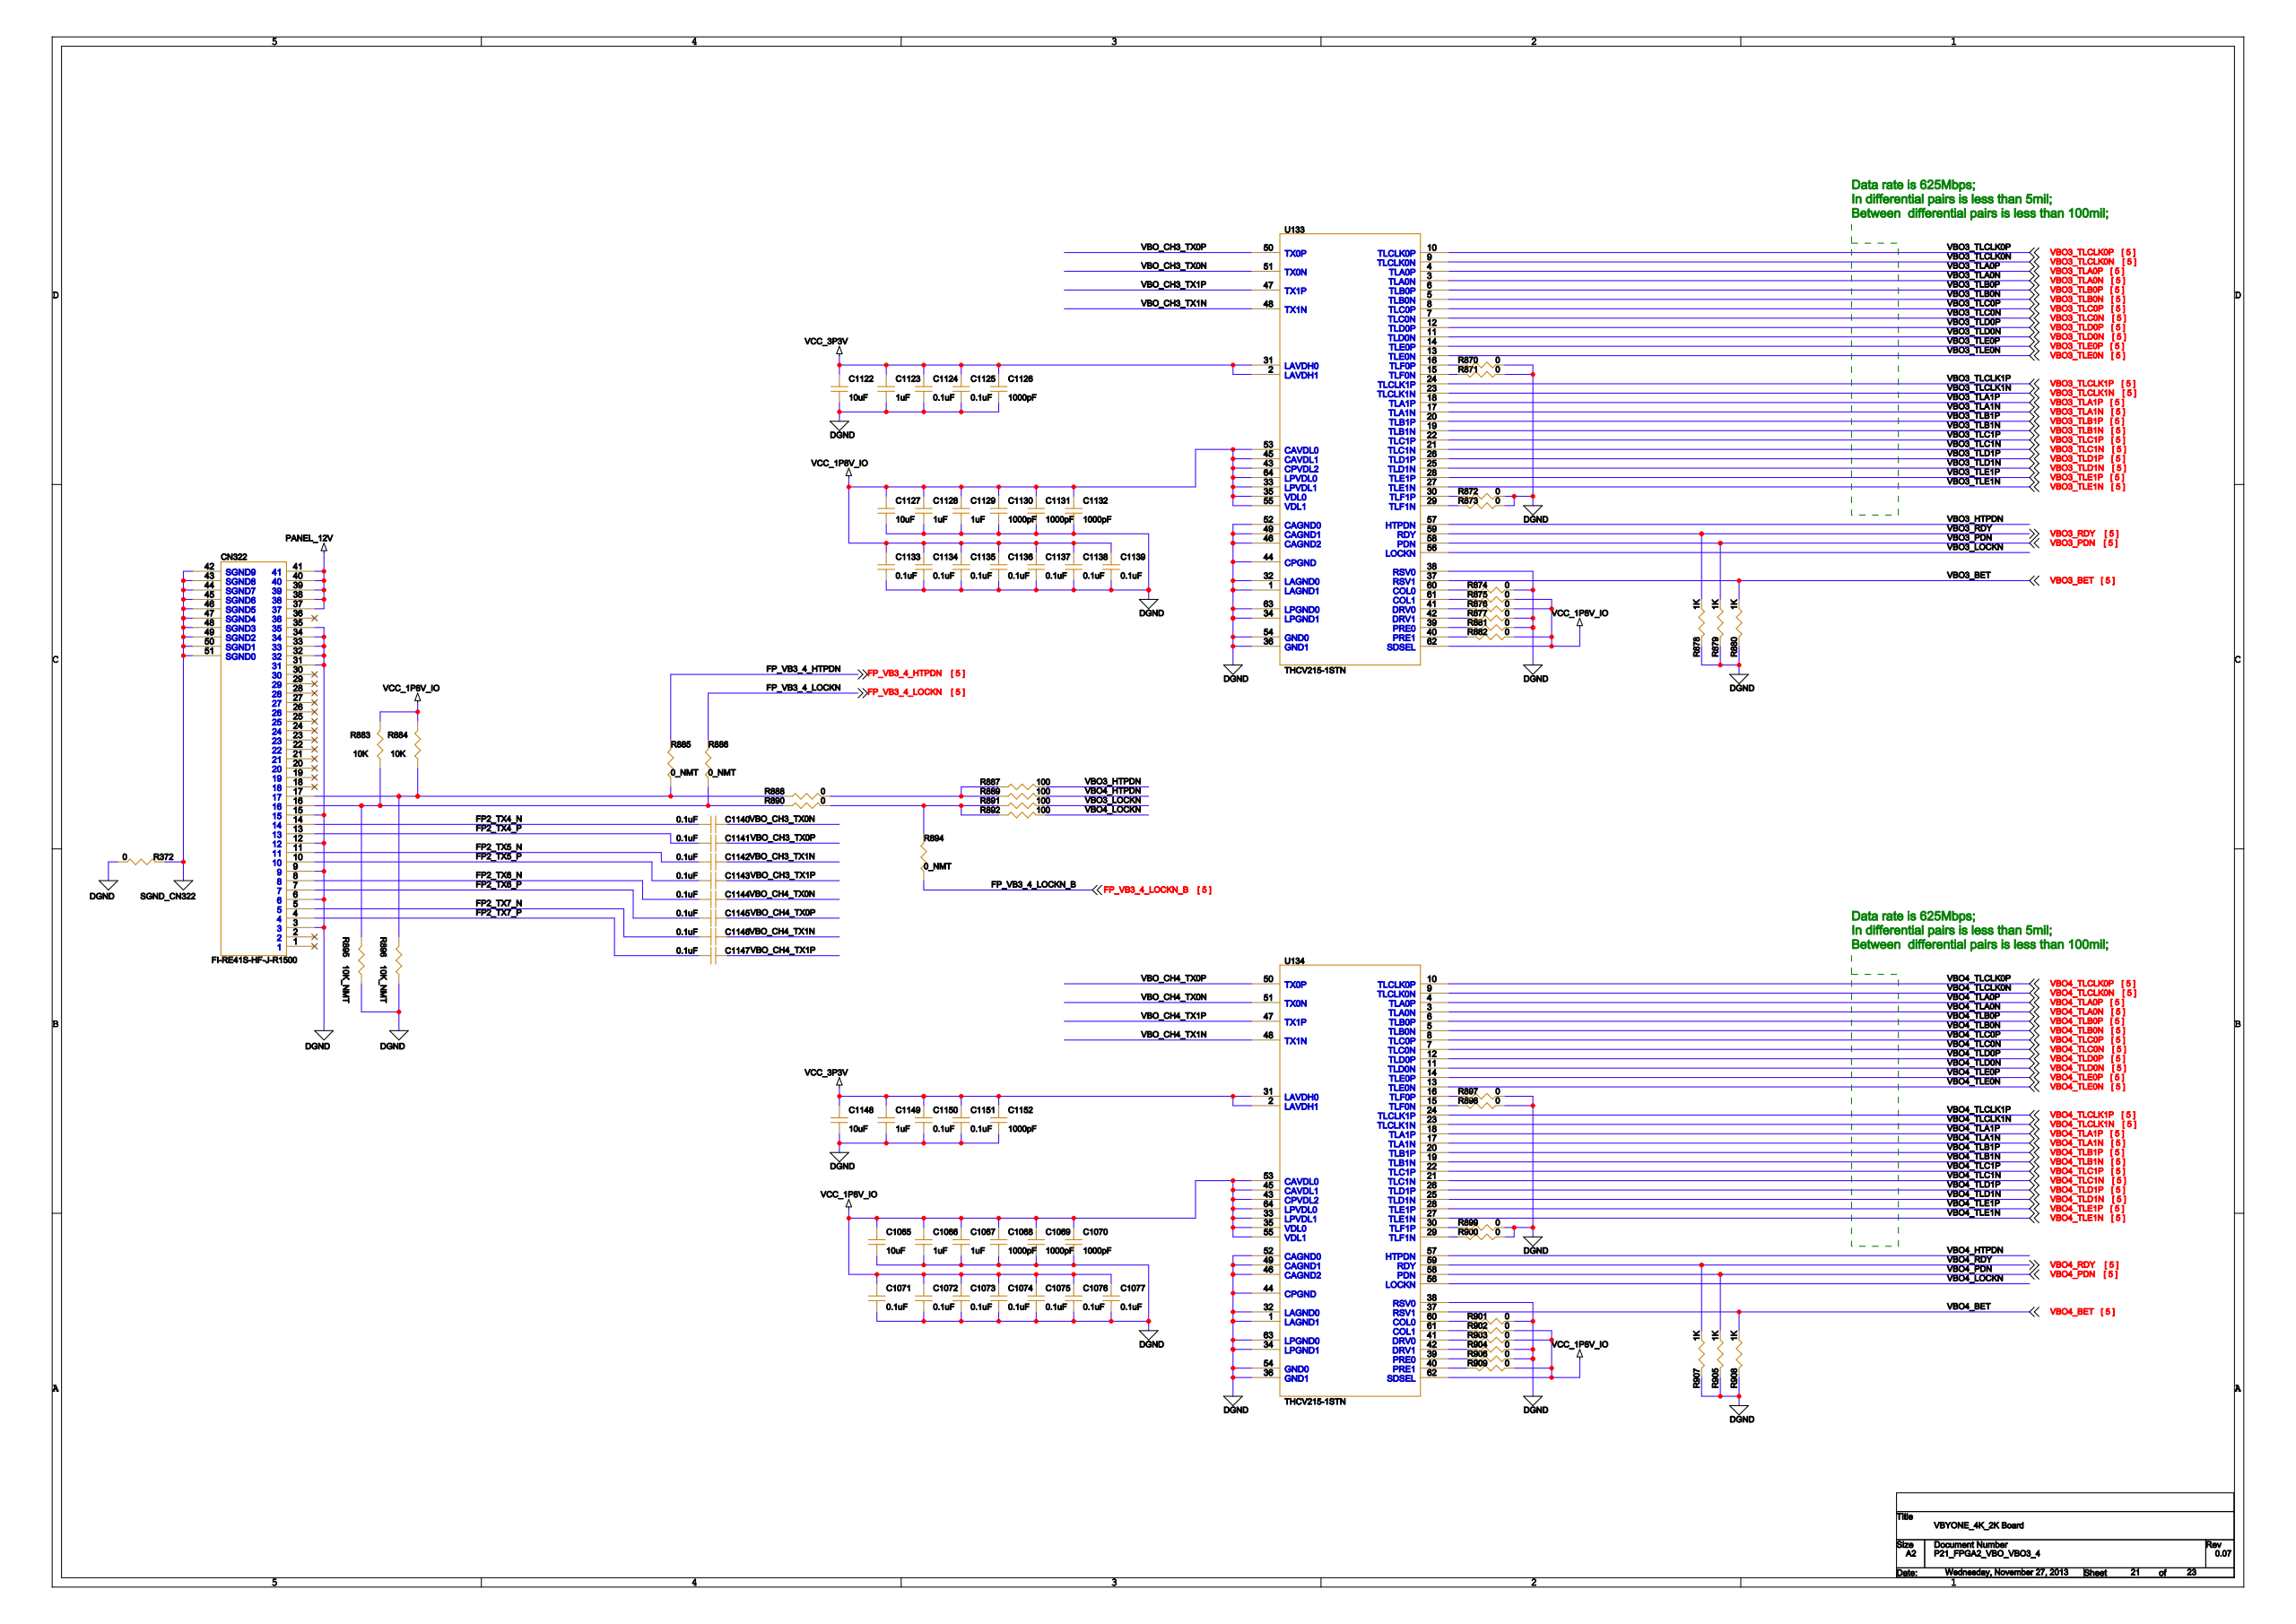Circuit board | Cadence Allegro | 1712 parts | 1495 nets | one sheet of the schematic
Parts on this sheet (reference | value | footprint):
C1065 | 10uF | CRC2012RZAS
C1066 | 1uF | CRC1608RZAS
C1067 | 1uF | CRC1608RZAS
C1068 | 1000pF | CRC1608RZAS
C1069 | 1000pF | CRC1608RZAS
C1070 | 1000pF | CRC1608RZAS
C1071 | 0.1uF | CRC1005RZAS
C1072 | 0.1uF | CRC1005RZAS
C1073 | 0.1uF | CRC1005RZAS
C1074 | 0.1uF | CRC1005RZAS
C1075 | 0.1uF | CRC1005RZAS
C1076 | 0.1uF | CRC1005RZAS
C1077 | 0.1uF | CRC1005RZAS
C1122 | 10uF | CRC2012RZAS
C1123 | 1uF | CRC1608RZAS
C1124 | 0.1uF | CRC1005RZAS
C1125 | 0.1uF | CRC1005RZAS
C1126 | 1000pF | CRC1608RZAS
C1127 | 10uF | CRC2012RZAS
C1128 | 1uF | CRC1608RZAS
C1129 | 1uF | CRC1608RZAS
C1130 | 1000pF | CRC1608RZAS
C1131 | 1000pF | CRC1608RZAS
C1132 | 1000pF | CRC1608RZAS
C1133 | 0.1uF | CRC1005RZAS
C1134 | 0.1uF | CRC1005RZAS
C1135 | 0.1uF | CRC1005RZAS
C1136 | 0.1uF | CRC1005RZAS
C1137 | 0.1uF | CRC1005RZAS
C1138 | 0.1uF | CRC1005RZAS
C1139 | 0.1uF | CRC1005RZAS
C1140 | 0.1uF | CRC1005RZAS
C1141 | 0.1uF | CRC1005RZAS
C1142 | 0.1uF | CRC1005RZAS
C1143 | 0.1uF | CRC1005RZAS
C1144 | 0.1uF | CRC1005RZAS
C1145 | 0.1uF | CRC1005RZAS
C1146 | 0.1uF | CRC1005RZAS
C1147 | 0.1uF | CRC1005RZAS
C1148 | 10uF | CRC2012RZAS
C1149 | 1uF | CRC1608RZAS
C1150 | 0.1uF | CRC1005RZAS
C1151 | 0.1uF | CRC1005RZAS
C1152 | 1000pF | CRC1608RZAS
CN322 | FI-RE41S-HF-J-R1500 | CAC041RCAS
R372 | 0 | CRC1608RZAS
R870 | 0 | CRC1608RZAS
R871 | 0 | CRC1608RZAS
R872 | 0 | CRC1608RZAS
R873 | 0 | CRC1608RZAS
R874 | 0 | CRC1608RZAS
R875 | 0 | CRC1608RZAS
R876 | 0 | CRC1608RZAS
R877 | 0 | CRC1608RZAS
R878 | 1K | CRC1608RZAS
R879 | 1K | CRC1608RZAS
R880 | 1K | CRC1608RZAS
R881 | 0 | CRC1608RZAS
R882 | 0 | CRC1608RZAS
R883 | 10K | CRC1005RZAS
R884 | 10K | CRC1005RZAS
R885 | 0_NMT | CRC1608RZAS
R886 | 0_NMT | CRC1608RZAS
R887 | 100 | CRC1005RZAS
R888 | 0 | CRC1608RZAS
R889 | 100 | CRC1005RZAS
R890 | 0 | CRC1608RZAS
R891 | 100 | CRC1005RZAS
R892 | 100 | CRC1005RZAS
R894 | 0_NMT | CRC1608RZAS
R895 | 10K_NMT | CRC1005RZAS
R896 | 10K_NMT | CRC1005RZAS
R897 | 0 | CRC1608RZAS
R898 | 0 | CRC1608RZAS
R899 | 0 | CRC1608RZAS
R900 | 0 | CRC1608RZAS
R901 | 0 | CRC1608RZAS
R902 | 0 | CRC1608RZAS
R903 | 0 | CRC1608RZAS
R904 | 0 | CRC1608RZAS
R905 | 1K | CRC1608RZAS
R906 | 0 | CRC1608RZAS
R907 | 1K | CRC1608RZAS
R908 | 1K | CRC1608RZAS
R909 | 0 | CRC1608RZAS
U133 | THCV215-1STN | SOC064RCAT
U134 | THCV215-1STN | SOC064RCAT
Nets of these parts (net: part-pin ...):
VCC_3P3V: C1122-2 C1123-2 C1124-2 C1125-2 C1126-2 C1148-2 C1149-2 C1150-2 C1151-2 C1152-2 U133-2 U133-31 U134-2 U134-31
DGND: C1065-1 C1066-1 C1067-1 C1068-1 C1069-1 C1070-1 C1071-1 C1072-1 C1073-1 C1074-1 C1075-1 C1076-1 C1077-1 C1122-1 C1123-1 C1124-1 C1125-1 C1126-1 C1127-1 C1128-1 C1129-1 C1130-1 C1131-1 C1132-1 C1133-1 C1134-1 C1135-1 C1136-1 C1137-1 C1138-1 C1139-1 C1148-1 C1149-1 C1150-1 C1151-1 C1152-1 R372-2 R870-2 R871-2 R872-2 R873-2 R874-2 R877-2 R878-1 R879-1 R880-1 R881-2 R895-2 R896-2 R897-2 R898-2 R899-2 R900-2 R901-2 R904-2 R905-1 R906-2 R907-1 R908-1 CN322-3 CN322-6 CN322-9 CN322-12 CN322-15 CN322-31 CN322-32 CN322-33 CN322-34 CN322-35 U133-1 U133-32 U133-34 U133-36 U133-38 U133-44 U133-46 U133-49 U133-52 U133-54 U133-63 U134-1 U134-32 U134-34 U134-36 U134-38 U134-44 U134-46 U134-49 U134-52 U134-54 U134-63
VCC_1P8V_IO: C1065-2 C1066-2 C1067-2 C1068-2 C1069-2 C1070-2 C1071-2 C1072-2 C1073-2 C1074-2 C1075-2 C1076-2 C1077-2 C1127-2 C1128-2 C1129-2 C1130-2 C1131-2 C1132-2 C1133-2 C1134-2 C1135-2 C1136-2 C1137-2 C1138-2 C1139-2 R875-2 R876-2 R882-2 R883-1 R884-1 R902-2 R903-2 R909-2 U133-33 U133-35 U133-43 U133-45 U133-53 U133-55 U133-62 U133-64 U134-33 U134-35 U134-43 U134-45 U134-53 U134-55 U134-62 U134-64
VBO_CH3_TX0N: C1140-1 U133-51
FP2_TX4_N: C1140-2 CN322-14
VBO_CH3_TX0P: C1141-1 U133-50
FP2_TX4_P: C1141-2 CN322-13
VBO_CH3_TX1N: C1142-1 U133-48
FP2_TX5_N: C1142-2 CN322-11
VBO_CH3_TX1P: C1143-1 U133-47
FP2_TX5_P: C1143-2 CN322-10
VBO_CH4_TX0N: C1144-1 U134-51
FP2_TX6_N: C1144-2 CN322-8
VBO_CH4_TX0P: C1145-1 U134-50
FP2_TX6_P: C1145-2 CN322-7
VBO_CH4_TX1N: C1146-1 U134-48
FP2_TX7_N: C1146-2 CN322-5
VBO_CH4_TX1P: C1147-1 U134-47
FP2_TX7_P: C1147-2 CN322-4
PANEL_12V: CN322-37 CN322-38 CN322-39 CN322-40 CN322-41
SGND_CN322: R372-1 CN322-42 CN322-43 CN322-44 CN322-45 CN322-46 CN322-47 CN322-48 CN322-49 CN322-50 CN322-51
N19766615: R883-2 R886-2 R890-2 R895-1 CN322-16
N19766613: R884-2 R885-2 R888-2 R896-1 CN322-17
N19766843: R887-2 R888-1 R889-2
N19766845: R890-1 R891-2 R892-2 R894-1
FP_VB3_4_HTPDN: R885-1
FP_VB3_4_LOCKN: R886-1
FP_VB3_4_LOCKN_B: R894-2
VBO3_HTPDN: R887-1 U133-57
VBO4_HTPDN: R889-1 U134-57
VBO3_LOCKN: R891-1 U133-56
VBO4_LOCKN: R892-1 U134-56
VBO3_RDY: R878-2 U133-59
VBO3_PDN: R879-2 U133-58
VBO3_BET: R880-2 U133-37
VBO4_PDN: R905-2 U134-58
VBO4_RDY: R907-2 U134-59
VBO4_BET: R908-2 U134-37
N19923475: R870-1 U133-16
N19923465: R871-1 U133-15
N19929189: R872-1 U133-30
N19929190: R873-1 U133-29
N20035029: R874-1 U133-60
N20035224: R875-1 U133-61
N19915968: R876-1 U133-41
N19915971: R877-1 U133-42
N19915974: R881-1 U133-39
N19915993: R882-1 U133-40
N19923368: R897-1 U134-16
N19923160: R898-1 U134-15
N19929972: R899-1 U134-30
N19929973: R900-1 U134-29
N20035671: R901-1 U134-60
N20035866: R902-1 U134-61
N19766087: R903-1 U134-41
N19766085: R904-1 U134-42
N19766093: R906-1 U134-39
N19766097: R909-1 U134-40
VBO3_TLC1P: U133-22
VBO3_TLA1P: U133-18
VBO3_TLA1N: U133-17
VBO3_TLA0P: U133-4
VBO3_TLA0N: U133-3
VBO4_TLD0P: U134-12
VBO3_TLC1N: U133-21
VBO3_TLC0P: U133-8
VBO3_TLC0N: U133-7
VBO3_TLD0P: U133-12
VBO3_TLD0N: U133-11
VBO4_TLD0N: U134-11
VBO3_TLE0P: U133-14
VBO3_TLE0N: U133-13
VBO3_TLCLK1P: U133-24
VBO3_TLCLK1N: U133-23
VBO3_TLB0P: U133-6
VBO4_TLC0P: U134-8
VBO3_TLCLK0P: U133-10
VBO3_TLCLK0N: U133-9
VBO3_TLB1P: U133-20
VBO3_TLB1N: U133-19
VBO3_TLB0N: U133-5
VBO4_TLC0N: U134-7
VBO4_TLCLK0P: U134-10
VBO4_TLCLK0N: U134-9
VBO4_TLA0P: U134-4
VBO4_TLA0N: U134-3
VBO3_TLD1P: U133-26
VBO3_TLD1N: U133-25
VBO4_TLB0P: U134-6
VBO4_TLB0N: U134-5
VBO4_TLE0P: U134-14
VBO4_TLE0N: U134-13
VBO3_TLE1P: U133-28
VBO3_TLE1N: U133-27
VBO4_TLD1P: U134-26
VBO4_TLA1P: U134-18
VBO4_TLCLK1P: U134-24
VBO4_TLC1P: U134-22
VBO4_TLC1N: U134-21
VBO4_TLE1P: U134-28
VBO4_TLE1N: U134-27
VBO4_TLD1N: U134-25
VBO4_TLA1N: U134-17
VBO4_TLCLK1N: U134-23
VBO4_TLB1P: U134-20
VBO4_TLB1N: U134-19